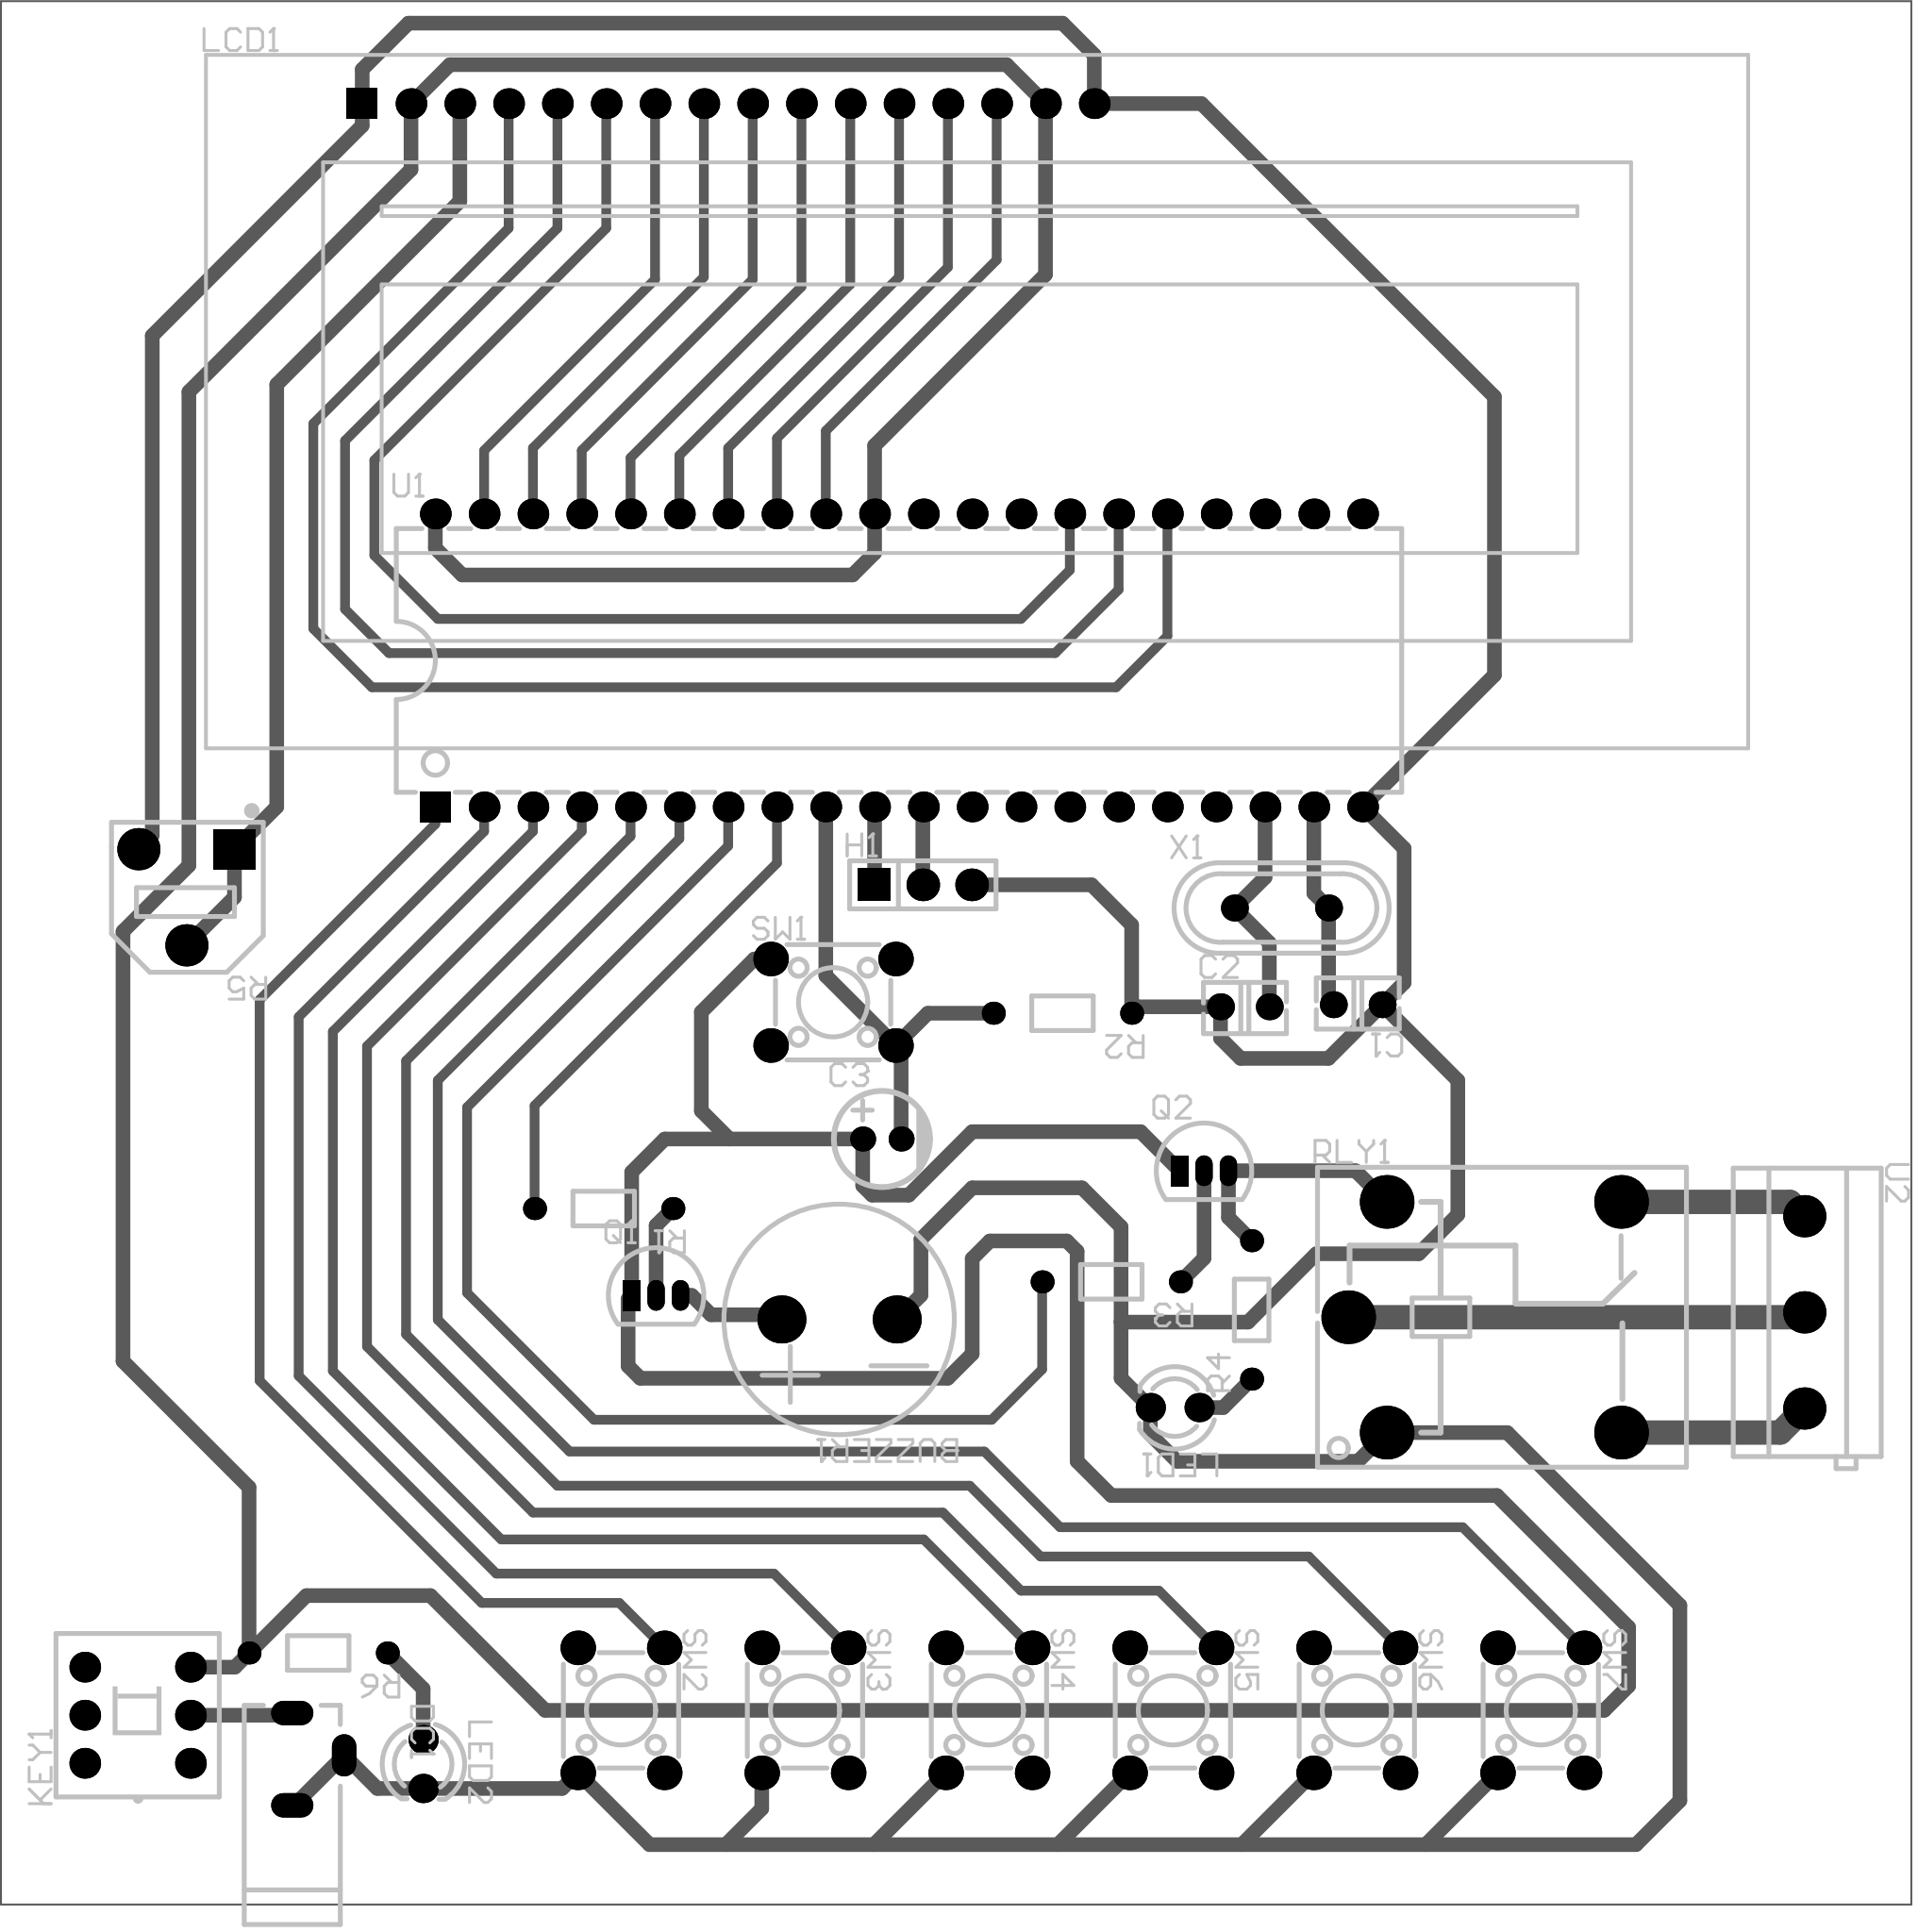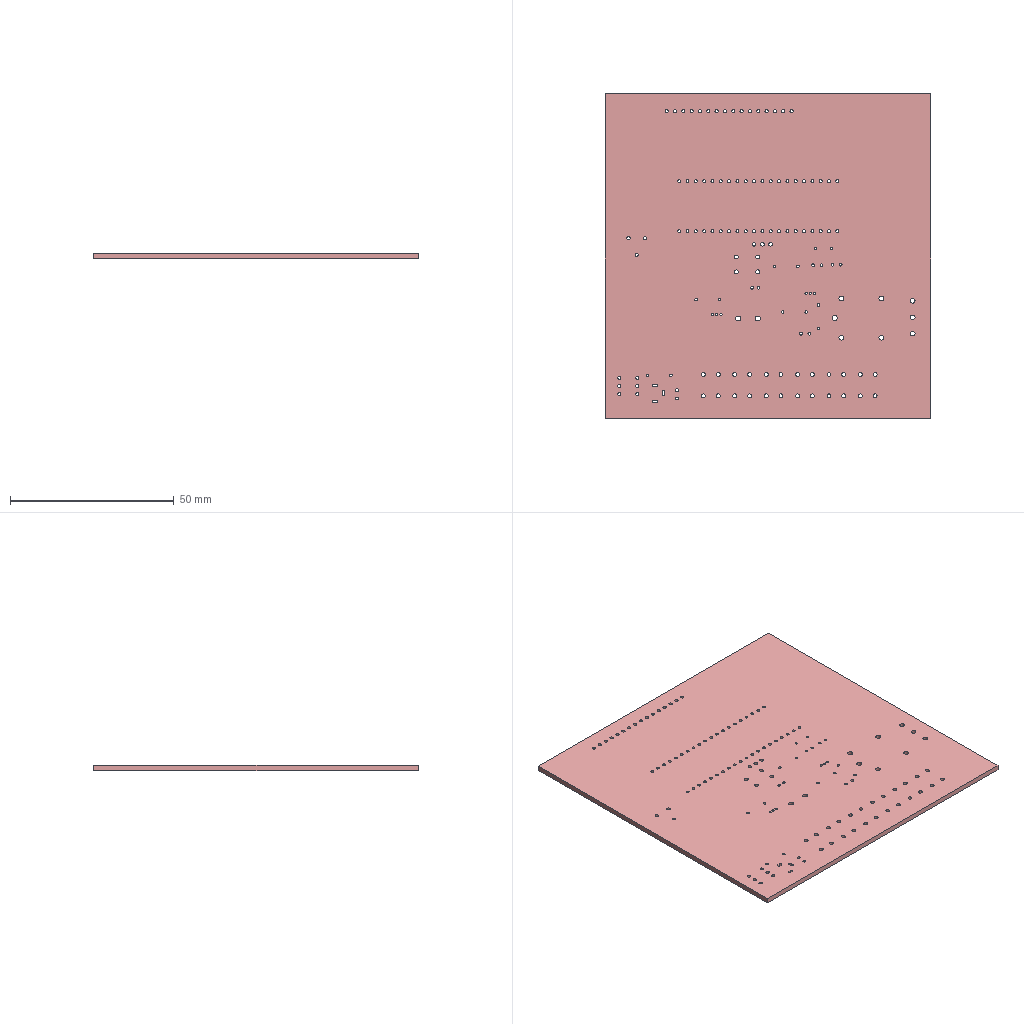Circuit board layout | Altium Designer | box 99.4 x 99 x 1.6 mm
Layer stack:
# Altium Designer layer stack of  (unit mm; dielectric type: 0 none, 1 core, 2 prepreg, 3 surface material)
index,name,kind,layer,copper_thickness_mm,dielectric_type,dielectric_thickness_mm,dielectric_material,dielectric_constant
0,Top Paste Mask Layer,other,,,,,,
1,Top Silkscreen Layer,other,,,,,,
2,Top Solder Mask Layer,dielectric,,,3,0.01,,3.3
3,Top Layer,copper,Top Layer,0.035,,,,
4,Dielectric1,dielectric,,,3,1.51,FR4,4.5
5,Bottom Layer,copper,Bottom Layer,0.035,,,,
6,Bottom Solder Mask Layer,dielectric,,,3,0.01,,3.3
7,Bottom Silkscreen Layer,other,,,,,,
8,Bottom Paste Mask Layer,other,,,,,,
# drill layer pairs: low layer,high layer
drill_pair,Top Layer,Bottom Layer
Part placement:
Designator,Comment,Layer,Footprint,Center-X(mm),Center-Y(mm),Rotation
BUZZER1,buzzer,TopLayer,BUZ-TH_BD12.0-P6.00-D0.9-RD,119.82,107.674,180
C1,30pF,TopLayer,CAP-TH_L3.8-W2.5-P2.54-D0.50,146.812,124.043,180
C2,30pF,TopLayer,CAP-TH_L3.8-W2.5-P2.54-D0.50,140.94,123.934,0
C3,10uF,TopLayer,CAP-TH_BD5.0-P2.00-D0.8-FD-10UF50VC110GL,122.047,117.058,0
H1,,TopLayer,HDR-TH_3P-P2.54-V-M,124.176,130.278,0
KEY1,无自锁开关 8.5×8.5 无声,TopLayer,SW-TH_6P-L8.5-W8.5-P2.54,83.312,87.086,90
LCD1,HS1602A,TopLayer,LCD1602,114.05,170.912,0
LED1,,TopLayer,LED_TH-3mm,137.287,103.088,180
LED2,,TopLayer,LED_TH-3mm,98.171,84.546,270
Q1,,TopLayer,S8550P_TO-92,110.295,108.924,0
Q2,,TopLayer,S8550P_TO-92,138.811,115.407,0
R1,1kΩ,TopLayer,Res_1/8W,107.569,113.439,180
R2,10kΩ,TopLayer,Res_1/8W,131.445,123.599,180
R3,1kΩ,TopLayer,Res_1/8W,133.985,109.629,180
R4,1kΩ,TopLayer,Res_1/8W,141.288,108.168,90
R5,10kΩ,TopLayer,RES-ADJ-SMD_RM065-V1,85.852,129.631,180
R6,1kΩ,TopLayer,Res_1/8W,92.71,90.325,180
RLY1,SRD-05VDC-SL-C,TopLayer,RELAY-TH_SRD-XXVDC-XL-C,153.416,107.787,0
SW1,,TopLayer,SW-TH_4P-L6.0-W6.0-P4.50-LS6.5,119.507,124.17,0
SW2,,TopLayer,SW-TH_4P-L6.0-W6.0-P4.50-LS6.5,108.47,87.34,270
SW3,,TopLayer,SW-TH_4P-L6.0-W6.0-P4.50-LS6.5,118.043,87.34,270
SW4,,TopLayer,SW-TH_4P-L6.0-W6.0-P4.50-LS6.5,127.617,87.34,270
SW5,,TopLayer,SW-TH_4P-L6.0-W6.0-P4.50-LS6.5,137.19,87.34,270
SW6,,TopLayer,SW-TH_4P-L6.0-W6.0-P4.50-LS6.5,146.764,87.34,270
SW7,,TopLayer,SW-TH_4P-L6.0-W6.0-P4.50-LS6.5,156.337,87.34,270
U1,STC89C52RC-40I-PDIP40,TopLayer,DIP-40_L52.0-W13.7-P2.54-LS15.2-BL,122.936,141.95,0
U2,KF301-5.0-3P,TopLayer,CONN-TH_3P-P5.00_KF301-5.0-3P,170.053,108.041,270
X1,11.059MHz,TopLayer,OSC-TH_L11.1-W4.7-P4.88,142.845,129.073,0
DC1,DC-002,TopLayer,DC-IN-TH_DC-3510,92.71,84.8,270
Pad and via stacks:
# Altium Designer via and pad stacks of  (unit mm). Each distinct definition once, with the count of objects using it.
# via: kind,start_layer,end_layer,hole_mm,diameter_mm,mode(0 simple;1 top-mid-bottom;2 full stack),diameter_per_layer,count,example_net
# pad: kind,layer,hole_mm,hole_type(0 round;1 square;2 slot),plating,top_size,top_shape(1 round;2 rect;3 octagon;9 rounded rect),mid_size,bottom_size,mode,footprint,size_per_layer,count,example
pad,Multi-Layer,1.5,0,plated,2.5x2.5,1,2.5x2.5,2.5x2.5,0,BUZ-TH_BD12.0-P6.00-D0.9-RD,,2,BUZZER1.1
pad,Multi-Layer,0.8,0,plated,1.4x1.4,1,1.4x1.4,1.4x1.4,0,CAP-TH_L3.8-W2.5-P2.54-D0.50,,4,C1.1
pad,Multi-Layer,0.8,0,plated,1.3x1.3,1,1.3x1.3,1.3x1.3,0,CAP-TH_BD5.0-P2.00-D0.8-FD-10UF50VC110GL,,2,C3.2
pad,Multi-Layer,1.1,0,plated,1.7x1.7,2,1.7x1.7,1.7x1.7,0,HDR-TH_3P-P2.54-V-M,,1,H1.1
pad,Multi-Layer,1.1,0,plated,1.7x1.7,1,1.7x1.7,1.7x1.7,0,HDR-TH_3P-P2.54-V-M,,2,H1.2
pad,Multi-Layer,1,0,plated,1.6x1.6,1,1.6x1.6,1.6x1.6,0,SW-TH_6P-L8.5-W8.5-P2.54,,6,KEY1.4
pad,Multi-Layer,1,0,plated,1.6x1.6,1,1.6x1.6,1.6x1.6,0,LCD1602,,15,LCD1.16
pad,Multi-Layer,1,0,plated,1.6x1.6,2,1.6x1.6,1.6x1.6,0,LCD1602,,1,LCD1.1
pad,Multi-Layer,0.9144,0,plated,1.524x1.524,1,1.524x1.524,1.524x1.524,0,LED_TH-3mm,,4,LED1.1
pad,Multi-Layer,0.7,0,plated,0.9x1.6,1,0.9x1.6,0.9x1.6,0,S8550P_TO-92,,4,Q1.3
pad,Multi-Layer,0.7,0,plated,0.9x1.6,2,0.9x1.6,0.9x1.6,0,S8550P_TO-92,,2,Q1.1
pad,Multi-Layer,0.8001,0,plated,1.199x1.199,1,1.199x1.199,1.199x1.199,0,Res_1/8W,,10,R1.1
pad,Multi-Layer,1,0,plated,2.2x2.1,2,2.2x2.1,2.2x2.1,0,RES-ADJ-SMD_RM065-V1,,1,R5.1
pad,Multi-Layer,1,0,plated,2.2x2.2,1,2.2x2.2,2.2x2.2,0,RES-ADJ-SMD_RM065-V1,,2,R5.3
pad,Multi-Layer,1.524,0,plated,2.794x2.794,1,2.794x2.794,2.794x2.794,0,RELAY-TH_SRD-XXVDC-XL-C,,5,RLY1.2
pad,Multi-Layer,1.2,0,plated,1.8x1.8,1,1.8x1.8,1.8x1.8,0,SW-TH_4P-L6.0-W6.0-P4.50-LS6.5,,28,SW1.1
pad,Multi-Layer,0.889,0,plated,1.6x1.6,1,1.6x1.6,1.6x1.6,0,DIP-40_L52.0-W13.7-P2.54-LS15.2-BL,,39,U1.31
pad,Multi-Layer,0.889,0,plated,1.6x1.6,2,1.6x1.6,1.6x1.6,0,DIP-40_L52.0-W13.7-P2.54-LS15.2-BL,,1,U1.1
pad,Multi-Layer,1.4,0,plated,2.2x2.2,1,2.2x2.2,2.2x2.2,0,CONN-TH_3P-P5.00_KF301-5.0-3P,,3,U2.1
pad,Multi-Layer,0.7,0,plated,1.4x1.4,1,1.4x1.4,1.4x1.4,0,OSC-TH_L11.1-W4.7-P4.88,,2,X1.1
pad,Multi-Layer,0.8,2,plated,2.2x1.27,1,2.2x1.27,2.2x1.27,0,DC-IN-TH_DC-3510,,3,DC1.3
Design rules, without the lines most boards share:
# Altium Designer design rules of  (exported by Altium Designer, unit mm)
# columns: name | kind | enabled | priority | scope1 | scope2 | descriptor | typed fields (field=value)
creepage | 65 | enabled | 1 | All | All | Creepage Distance Constraint =(0mil) (All),(All) |